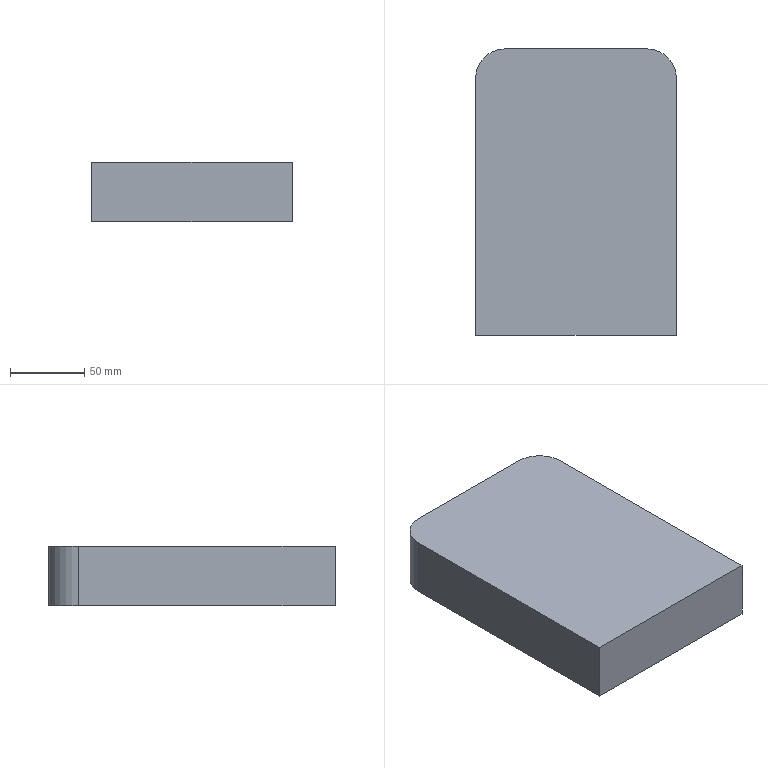Part | SolidWorks | features Extrusion 1, Shell 1 | 1 solid | 15 faces | box 135.332 x 192.723 x 40 mm | volume 238240 mm3 | plane 11 | cylinder 4 | commonest cylinder face diameters 30 x2 40 x2
STEP:
#1=CARTESIAN_POINT('',(-11.593,120.781,0.));
#2=VERTEX_POINT('',#1);
#3=CARTESIAN_POINT('',(-11.593,-51.942,0.));
#4=VERTEX_POINT('',#3);
#5=CARTESIAN_POINT('',(-11.593,120.781,0.));
#6=DIRECTION('',(0.,-1.,0.));
#7=VECTOR('',#6,1000.);
#8=LINE('',#5,#7);
#9=EDGE_CURVE('',#2,#4,#8,.T.);
#10=ORIENTED_EDGE('',*,*,#9,.T.);
#11=CARTESIAN_POINT('',(-11.593,-51.942,40.));
#12=VERTEX_POINT('',#11);
#13=CARTESIAN_POINT('',(-11.593,-51.942,40.));
#14=DIRECTION('',(0.,0.,-1.));
#15=VECTOR('',#14,1000.);
#16=LINE('',#13,#15);
#17=EDGE_CURVE('',#12,#4,#16,.T.);
#18=ORIENTED_EDGE('',*,*,#17,.F.);
#19=CARTESIAN_POINT('',(-11.593,120.781,40.));
#20=VERTEX_POINT('',#19);
#21=CARTESIAN_POINT('',(-11.593,120.781,40.));
#22=DIRECTION('',(0.,-1.,0.));
#23=VECTOR('',#22,1000.);
#24=LINE('',#21,#23);
#25=EDGE_CURVE('',#20,#12,#24,.T.);
#26=ORIENTED_EDGE('',*,*,#25,.F.);
#27=CARTESIAN_POINT('',(-11.593,120.781,40.));
#28=DIRECTION('',(0.,0.,-1.));
#29=VECTOR('',#28,1000.);
#30=LINE('',#27,#29);
#31=EDGE_CURVE('',#20,#2,#30,.T.);
#32=ORIENTED_EDGE('',*,*,#31,.T.);
#33=EDGE_LOOP('',(#10,#18,#26,#32));
#34=FACE_OUTER_BOUND('',#33,.T.);
#35=CARTESIAN_POINT('',(-11.593,120.781,40.));
#36=DIRECTION('',(1.,0.,0.));
#37=DIRECTION('',(0.,1.,0.));
#38=AXIS2_PLACEMENT_3D('',#35,#36,#37);
#39=PLANE('',#38);
#40=ADVANCED_FACE('',(#34),#39,.F.);
#41=CARTESIAN_POINT('',(123.739,-51.942,0.));
#42=VERTEX_POINT('',#41);
#43=CARTESIAN_POINT('',(92.171,-51.942,0.));
#44=DIRECTION('',(1.,0.,0.));
#45=VECTOR('',#44,1000.);
#46=LINE('',#43,#45);
#47=EDGE_CURVE('',#4,#42,#46,.T.);
#48=ORIENTED_EDGE('',*,*,#47,.T.);
#49=CARTESIAN_POINT('',(123.739,-51.942,40.));
#50=VERTEX_POINT('',#49);
#51=CARTESIAN_POINT('',(123.739,-51.942,40.));
#52=DIRECTION('',(0.,0.,-1.));
#53=VECTOR('',#52,1000.);
#54=LINE('',#51,#53);
#55=EDGE_CURVE('',#50,#42,#54,.T.);
#56=ORIENTED_EDGE('',*,*,#55,.F.);
#57=CARTESIAN_POINT('',(-11.593,-51.942,40.));
#58=DIRECTION('',(1.,0.,0.));
#59=VECTOR('',#58,1000.);
#60=LINE('',#57,#59);
#61=EDGE_CURVE('',#12,#50,#60,.T.);
#62=ORIENTED_EDGE('',*,*,#61,.F.);
#63=ORIENTED_EDGE('',*,*,#17,.T.);
#64=EDGE_LOOP('',(#48,#56,#62,#63));
#65=FACE_OUTER_BOUND('',#64,.T.);
#66=CARTESIAN_POINT('',(92.171,-51.942,40.));
#67=DIRECTION('',(0.,1.,0.));
#68=DIRECTION('',(0.,0.,1.));
#69=AXIS2_PLACEMENT_3D('',#66,#67,#68);
#70=PLANE('',#69);
#71=ADVANCED_FACE('',(#65),#70,.F.);
#72=CARTESIAN_POINT('',(123.739,120.781,0.));
#73=VERTEX_POINT('',#72);
#74=CARTESIAN_POINT('',(123.739,-51.942,0.));
#75=DIRECTION('',(0.,1.,0.));
#76=VECTOR('',#75,1000.);
#77=LINE('',#74,#76);
#78=EDGE_CURVE('',#42,#73,#77,.T.);
#79=ORIENTED_EDGE('',*,*,#78,.T.);
#80=CARTESIAN_POINT('',(123.739,120.781,40.));
#81=VERTEX_POINT('',#80);
#82=CARTESIAN_POINT('',(123.739,120.781,40.));
#83=DIRECTION('',(0.,0.,-1.));
#84=VECTOR('',#83,1000.);
#85=LINE('',#82,#84);
#86=EDGE_CURVE('',#81,#73,#85,.T.);
#87=ORIENTED_EDGE('',*,*,#86,.F.);
#88=CARTESIAN_POINT('',(123.739,-51.942,40.));
#89=DIRECTION('',(0.,1.,0.));
#90=VECTOR('',#89,1000.);
#91=LINE('',#88,#90);
#92=EDGE_CURVE('',#50,#81,#91,.T.);
#93=ORIENTED_EDGE('',*,*,#92,.F.);
#94=ORIENTED_EDGE('',*,*,#55,.T.);
#95=EDGE_LOOP('',(#79,#87,#93,#94));
#96=FACE_OUTER_BOUND('',#95,.T.);
#97=CARTESIAN_POINT('',(123.739,-51.942,40.));
#98=DIRECTION('',(-1.,0.,0.));
#99=DIRECTION('',(0.,-1.,0.));
#100=AXIS2_PLACEMENT_3D('',#97,#98,#99);
#101=PLANE('',#100);
#102=ADVANCED_FACE('',(#96),#101,.F.);
#103=CARTESIAN_POINT('',(103.739,140.781,0.));
#104=VERTEX_POINT('',#103);
#105=CARTESIAN_POINT('',(103.739,120.781,0.));
#106=DIRECTION('',(0.,0.,1.));
#107=DIRECTION('',(1.,0.,0.));
#108=AXIS2_PLACEMENT_3D('',#105,#106,#107);
#109=CIRCLE('',#108,20.);
#110=EDGE_CURVE('',#73,#104,#109,.T.);
#111=ORIENTED_EDGE('',*,*,#110,.T.);
#112=CARTESIAN_POINT('',(103.739,140.781,40.));
#113=VERTEX_POINT('',#112);
#114=CARTESIAN_POINT('',(103.739,140.781,40.));
#115=DIRECTION('',(0.,0.,-1.));
#116=VECTOR('',#115,1000.);
#117=LINE('',#114,#116);
#118=EDGE_CURVE('',#113,#104,#117,.T.);
#119=ORIENTED_EDGE('',*,*,#118,.F.);
#120=CARTESIAN_POINT('',(103.739,120.781,40.));
#121=DIRECTION('',(0.,0.,1.));
#122=DIRECTION('',(1.,0.,0.));
#123=AXIS2_PLACEMENT_3D('',#120,#121,#122);
#124=CIRCLE('',#123,20.);
#125=EDGE_CURVE('',#81,#113,#124,.T.);
#126=ORIENTED_EDGE('',*,*,#125,.F.);
#127=ORIENTED_EDGE('',*,*,#86,.T.);
#128=EDGE_LOOP('',(#111,#119,#126,#127));
#129=FACE_OUTER_BOUND('',#128,.T.);
#130=CARTESIAN_POINT('',(103.739,120.781,40.));
#131=DIRECTION('',(0.,0.,-1.));
#132=DIRECTION('',(-1.,0.,0.));
#133=AXIS2_PLACEMENT_3D('',#130,#131,#132);
#134=CYLINDRICAL_SURFACE('',#133,20.);
#135=ADVANCED_FACE('',(#129),#134,.T.);
#136=CARTESIAN_POINT('',(8.407,140.781,0.));
#137=VERTEX_POINT('',#136);
#138=CARTESIAN_POINT('',(103.739,140.781,0.));
#139=DIRECTION('',(-1.,0.,0.));
#140=VECTOR('',#139,1000.);
#141=LINE('',#138,#140);
#142=EDGE_CURVE('',#104,#137,#141,.T.);
#143=ORIENTED_EDGE('',*,*,#142,.T.);
#144=CARTESIAN_POINT('',(8.407,140.781,40.));
#145=VERTEX_POINT('',#144);
#146=CARTESIAN_POINT('',(8.407,140.781,40.));
#147=DIRECTION('',(0.,0.,-1.));
#148=VECTOR('',#147,1000.);
#149=LINE('',#146,#148);
#150=EDGE_CURVE('',#145,#137,#149,.T.);
#151=ORIENTED_EDGE('',*,*,#150,.F.);
#152=CARTESIAN_POINT('',(103.739,140.781,40.));
#153=DIRECTION('',(-1.,0.,0.));
#154=VECTOR('',#153,1000.);
#155=LINE('',#152,#154);
#156=EDGE_CURVE('',#113,#145,#155,.T.);
#157=ORIENTED_EDGE('',*,*,#156,.F.);
#158=ORIENTED_EDGE('',*,*,#118,.T.);
#159=EDGE_LOOP('',(#143,#151,#157,#158));
#160=FACE_OUTER_BOUND('',#159,.T.);
#161=CARTESIAN_POINT('',(103.739,140.781,40.));
#162=DIRECTION('',(0.,-1.,0.));
#163=DIRECTION('',(0.,0.,-1.));
#164=AXIS2_PLACEMENT_3D('',#161,#162,#163);
#165=PLANE('',#164);
#166=ADVANCED_FACE('',(#160),#165,.F.);
#167=CARTESIAN_POINT('',(8.407,120.781,0.));
#168=DIRECTION('',(0.,0.,1.));
#169=DIRECTION('',(1.,0.,0.));
#170=AXIS2_PLACEMENT_3D('',#167,#168,#169);
#171=CIRCLE('',#170,20.);
#172=EDGE_CURVE('',#137,#2,#171,.T.);
#173=ORIENTED_EDGE('',*,*,#172,.T.);
#174=ORIENTED_EDGE('',*,*,#31,.F.);
#175=CARTESIAN_POINT('',(8.407,120.781,40.));
#176=DIRECTION('',(0.,0.,1.));
#177=DIRECTION('',(1.,0.,0.));
#178=AXIS2_PLACEMENT_3D('',#175,#176,#177);
#179=CIRCLE('',#178,20.);
#180=EDGE_CURVE('',#145,#20,#179,.T.);
#181=ORIENTED_EDGE('',*,*,#180,.F.);
#182=ORIENTED_EDGE('',*,*,#150,.T.);
#183=EDGE_LOOP('',(#173,#174,#181,#182));
#184=FACE_OUTER_BOUND('',#183,.T.);
#185=CARTESIAN_POINT('',(8.407,120.781,40.));
#186=DIRECTION('',(0.,0.,-1.));
#187=DIRECTION('',(-1.,0.,0.));
#188=AXIS2_PLACEMENT_3D('',#185,#186,#187);
#189=CYLINDRICAL_SURFACE('',#188,20.);
#190=ADVANCED_FACE('',(#184),#189,.T.);
#191=ORIENTED_EDGE('',*,*,#25,.T.);
#192=ORIENTED_EDGE('',*,*,#61,.T.);
#193=ORIENTED_EDGE('',*,*,#92,.T.);
#194=ORIENTED_EDGE('',*,*,#125,.T.);
#195=ORIENTED_EDGE('',*,*,#156,.T.);
#196=ORIENTED_EDGE('',*,*,#180,.T.);
#197=EDGE_LOOP('',(#191,#192,#193,#194,#195,#196));
#198=FACE_OUTER_BOUND('',#197,.T.);
#199=CARTESIAN_POINT('',(103.739,120.781,40.));
#200=DIRECTION('',(0.,0.,1.));
#201=DIRECTION('',(1.,0.,0.));
#202=AXIS2_PLACEMENT_3D('',#199,#200,#201);
#203=PLANE('',#202);
#204=ADVANCED_FACE('',(#198),#203,.T.);
#205=CARTESIAN_POINT('',(8.407,135.781,0.));
#206=VERTEX_POINT('',#205);
#207=CARTESIAN_POINT('',(-6.593,120.781,0.));
#208=VERTEX_POINT('',#207);
#209=CARTESIAN_POINT('',(8.407,120.781,0.));
#210=DIRECTION('',(0.,0.,1.));
#211=DIRECTION('',(1.,0.,0.));
#212=AXIS2_PLACEMENT_3D('',#209,#210,#211);
#213=CIRCLE('',#212,15.);
#214=EDGE_CURVE('',#206,#208,#213,.T.);
#215=ORIENTED_EDGE('',*,*,#214,.T.);
#216=CARTESIAN_POINT('',(-6.593,-46.942,0.));
#217=VERTEX_POINT('',#216);
#218=CARTESIAN_POINT('',(-6.593,120.781,0.));
#219=DIRECTION('',(0.,-1.,0.));
#220=VECTOR('',#219,1000.);
#221=LINE('',#218,#220);
#222=EDGE_CURVE('',#208,#217,#221,.T.);
#223=ORIENTED_EDGE('',*,*,#222,.T.);
#224=CARTESIAN_POINT('',(118.739,-46.942,0.));
#225=VERTEX_POINT('',#224);
#226=CARTESIAN_POINT('',(92.171,-46.942,0.));
#227=DIRECTION('',(1.,0.,0.));
#228=VECTOR('',#227,1000.);
#229=LINE('',#226,#228);
#230=EDGE_CURVE('',#217,#225,#229,.T.);
#231=ORIENTED_EDGE('',*,*,#230,.T.);
#232=CARTESIAN_POINT('',(118.739,120.781,0.));
#233=VERTEX_POINT('',#232);
#234=CARTESIAN_POINT('',(118.739,-51.942,0.));
#235=DIRECTION('',(0.,1.,0.));
#236=VECTOR('',#235,1000.);
#237=LINE('',#234,#236);
#238=EDGE_CURVE('',#225,#233,#237,.T.);
#239=ORIENTED_EDGE('',*,*,#238,.T.);
#240=CARTESIAN_POINT('',(103.739,135.781,0.));
#241=VERTEX_POINT('',#240);
#242=CARTESIAN_POINT('',(103.739,120.781,0.));
#243=DIRECTION('',(0.,0.,1.));
#244=DIRECTION('',(1.,0.,0.));
#245=AXIS2_PLACEMENT_3D('',#242,#243,#244);
#246=CIRCLE('',#245,15.);
#247=EDGE_CURVE('',#233,#241,#246,.T.);
#248=ORIENTED_EDGE('',*,*,#247,.T.);
#249=CARTESIAN_POINT('',(103.739,135.781,0.));
#250=DIRECTION('',(-1.,0.,0.));
#251=VECTOR('',#250,1000.);
#252=LINE('',#249,#251);
#253=EDGE_CURVE('',#241,#206,#252,.T.);
#254=ORIENTED_EDGE('',*,*,#253,.T.);
#255=EDGE_LOOP('',(#215,#223,#231,#239,#248,#254));
#256=FACE_BOUND('',#255,.T.);
#257=ORIENTED_EDGE('',*,*,#9,.F.);
#258=ORIENTED_EDGE('',*,*,#172,.F.);
#259=ORIENTED_EDGE('',*,*,#142,.F.);
#260=ORIENTED_EDGE('',*,*,#110,.F.);
#261=ORIENTED_EDGE('',*,*,#78,.F.);
#262=ORIENTED_EDGE('',*,*,#47,.F.);
#263=EDGE_LOOP('',(#257,#258,#259,#260,#261,#262));
#264=FACE_OUTER_BOUND('',#263,.T.);
#265=CARTESIAN_POINT('',(103.739,120.781,0.));
#266=DIRECTION('',(0.,0.,1.));
#267=DIRECTION('',(1.,0.,0.));
#268=AXIS2_PLACEMENT_3D('',#265,#266,#267);
#269=PLANE('',#268);
#270=ADVANCED_FACE('',(#256,#264),#269,.F.);
#271=ORIENTED_EDGE('',*,*,#222,.F.);
#272=CARTESIAN_POINT('',(-6.593,120.781,35.));
#273=VERTEX_POINT('',#272);
#274=CARTESIAN_POINT('',(-6.593,120.781,40.));
#275=DIRECTION('',(0.,0.,-1.));
#276=VECTOR('',#275,1000.);
#277=LINE('',#274,#276);
#278=EDGE_CURVE('',#273,#208,#277,.T.);
#279=ORIENTED_EDGE('',*,*,#278,.F.);
#280=CARTESIAN_POINT('',(-6.593,-46.942,35.));
#281=VERTEX_POINT('',#280);
#282=CARTESIAN_POINT('',(-6.593,120.781,35.));
#283=DIRECTION('',(0.,-1.,0.));
#284=VECTOR('',#283,1000.);
#285=LINE('',#282,#284);
#286=EDGE_CURVE('',#273,#281,#285,.T.);
#287=ORIENTED_EDGE('',*,*,#286,.T.);
#288=CARTESIAN_POINT('',(-6.593,-46.942,40.));
#289=DIRECTION('',(0.,0.,-1.));
#290=VECTOR('',#289,1000.);
#291=LINE('',#288,#290);
#292=EDGE_CURVE('',#281,#217,#291,.T.);
#293=ORIENTED_EDGE('',*,*,#292,.T.);
#294=EDGE_LOOP('',(#271,#279,#287,#293));
#295=FACE_OUTER_BOUND('',#294,.T.);
#296=CARTESIAN_POINT('',(-6.593,120.781,40.));
#297=DIRECTION('',(1.,0.,0.));
#298=DIRECTION('',(0.,1.,0.));
#299=AXIS2_PLACEMENT_3D('',#296,#297,#298);
#300=PLANE('',#299);
#301=ADVANCED_FACE('',(#295),#300,.T.);
#302=ORIENTED_EDGE('',*,*,#230,.F.);
#303=ORIENTED_EDGE('',*,*,#292,.F.);
#304=CARTESIAN_POINT('',(118.739,-46.942,35.));
#305=VERTEX_POINT('',#304);
#306=CARTESIAN_POINT('',(92.171,-46.942,35.));
#307=DIRECTION('',(1.,0.,0.));
#308=VECTOR('',#307,1000.);
#309=LINE('',#306,#308);
#310=EDGE_CURVE('',#281,#305,#309,.T.);
#311=ORIENTED_EDGE('',*,*,#310,.T.);
#312=CARTESIAN_POINT('',(118.739,-46.942,40.));
#313=DIRECTION('',(0.,0.,-1.));
#314=VECTOR('',#313,1000.);
#315=LINE('',#312,#314);
#316=EDGE_CURVE('',#305,#225,#315,.T.);
#317=ORIENTED_EDGE('',*,*,#316,.T.);
#318=EDGE_LOOP('',(#302,#303,#311,#317));
#319=FACE_OUTER_BOUND('',#318,.T.);
#320=CARTESIAN_POINT('',(92.171,-46.942,40.));
#321=DIRECTION('',(0.,1.,0.));
#322=DIRECTION('',(0.,0.,1.));
#323=AXIS2_PLACEMENT_3D('',#320,#321,#322);
#324=PLANE('',#323);
#325=ADVANCED_FACE('',(#319),#324,.T.);
#326=ORIENTED_EDGE('',*,*,#238,.F.);
#327=ORIENTED_EDGE('',*,*,#316,.F.);
#328=CARTESIAN_POINT('',(118.739,120.781,35.));
#329=VERTEX_POINT('',#328);
#330=CARTESIAN_POINT('',(118.739,-51.942,35.));
#331=DIRECTION('',(0.,1.,0.));
#332=VECTOR('',#331,1000.);
#333=LINE('',#330,#332);
#334=EDGE_CURVE('',#305,#329,#333,.T.);
#335=ORIENTED_EDGE('',*,*,#334,.T.);
#336=CARTESIAN_POINT('',(118.739,120.781,40.));
#337=DIRECTION('',(0.,0.,-1.));
#338=VECTOR('',#337,1000.);
#339=LINE('',#336,#338);
#340=EDGE_CURVE('',#329,#233,#339,.T.);
#341=ORIENTED_EDGE('',*,*,#340,.T.);
#342=EDGE_LOOP('',(#326,#327,#335,#341));
#343=FACE_OUTER_BOUND('',#342,.T.);
#344=CARTESIAN_POINT('',(118.739,-51.942,40.));
#345=DIRECTION('',(-1.,0.,0.));
#346=DIRECTION('',(0.,-1.,0.));
#347=AXIS2_PLACEMENT_3D('',#344,#345,#346);
#348=PLANE('',#347);
#349=ADVANCED_FACE('',(#343),#348,.T.);
#350=ORIENTED_EDGE('',*,*,#247,.F.);
#351=ORIENTED_EDGE('',*,*,#340,.F.);
#352=CARTESIAN_POINT('',(103.739,135.781,35.));
#353=VERTEX_POINT('',#352);
#354=CARTESIAN_POINT('',(103.739,120.781,35.));
#355=DIRECTION('',(0.,0.,1.));
#356=DIRECTION('',(1.,0.,0.));
#357=AXIS2_PLACEMENT_3D('',#354,#355,#356);
#358=CIRCLE('',#357,15.);
#359=EDGE_CURVE('',#329,#353,#358,.T.);
#360=ORIENTED_EDGE('',*,*,#359,.T.);
#361=CARTESIAN_POINT('',(103.739,135.781,40.));
#362=DIRECTION('',(0.,0.,-1.));
#363=VECTOR('',#362,1000.);
#364=LINE('',#361,#363);
#365=EDGE_CURVE('',#353,#241,#364,.T.);
#366=ORIENTED_EDGE('',*,*,#365,.T.);
#367=EDGE_LOOP('',(#350,#351,#360,#366));
#368=FACE_OUTER_BOUND('',#367,.T.);
#369=CARTESIAN_POINT('',(103.739,120.781,40.));
#370=DIRECTION('',(0.,0.,-1.));
#371=DIRECTION('',(-1.,0.,0.));
#372=AXIS2_PLACEMENT_3D('',#369,#370,#371);
#373=CYLINDRICAL_SURFACE('',#372,15.);
#374=ADVANCED_FACE('',(#368),#373,.F.);
#375=ORIENTED_EDGE('',*,*,#253,.F.);
#376=ORIENTED_EDGE('',*,*,#365,.F.);
#377=CARTESIAN_POINT('',(8.407,135.781,35.));
#378=VERTEX_POINT('',#377);
#379=CARTESIAN_POINT('',(103.739,135.781,35.));
#380=DIRECTION('',(-1.,0.,0.));
#381=VECTOR('',#380,1000.);
#382=LINE('',#379,#381);
#383=EDGE_CURVE('',#353,#378,#382,.T.);
#384=ORIENTED_EDGE('',*,*,#383,.T.);
#385=CARTESIAN_POINT('',(8.407,135.781,40.));
#386=DIRECTION('',(0.,0.,-1.));
#387=VECTOR('',#386,1000.);
#388=LINE('',#385,#387);
#389=EDGE_CURVE('',#378,#206,#388,.T.);
#390=ORIENTED_EDGE('',*,*,#389,.T.);
#391=EDGE_LOOP('',(#375,#376,#384,#390));
#392=FACE_OUTER_BOUND('',#391,.T.);
#393=CARTESIAN_POINT('',(103.739,135.781,40.));
#394=DIRECTION('',(0.,-1.,0.));
#395=DIRECTION('',(0.,0.,-1.));
#396=AXIS2_PLACEMENT_3D('',#393,#394,#395);
#397=PLANE('',#396);
#398=ADVANCED_FACE('',(#392),#397,.T.);
#399=ORIENTED_EDGE('',*,*,#214,.F.);
#400=ORIENTED_EDGE('',*,*,#389,.F.);
#401=CARTESIAN_POINT('',(8.407,120.781,35.));
#402=DIRECTION('',(0.,0.,1.));
#403=DIRECTION('',(1.,0.,0.));
#404=AXIS2_PLACEMENT_3D('',#401,#402,#403);
#405=CIRCLE('',#404,15.);
#406=EDGE_CURVE('',#378,#273,#405,.T.);
#407=ORIENTED_EDGE('',*,*,#406,.T.);
#408=ORIENTED_EDGE('',*,*,#278,.T.);
#409=EDGE_LOOP('',(#399,#400,#407,#408));
#410=FACE_OUTER_BOUND('',#409,.T.);
#411=CARTESIAN_POINT('',(8.407,120.781,40.));
#412=DIRECTION('',(0.,0.,-1.));
#413=DIRECTION('',(-1.,0.,0.));
#414=AXIS2_PLACEMENT_3D('',#411,#412,#413);
#415=CYLINDRICAL_SURFACE('',#414,15.);
#416=ADVANCED_FACE('',(#410),#415,.F.);
#417=ORIENTED_EDGE('',*,*,#286,.F.);
#418=ORIENTED_EDGE('',*,*,#406,.F.);
#419=ORIENTED_EDGE('',*,*,#383,.F.);
#420=ORIENTED_EDGE('',*,*,#359,.F.);
#421=ORIENTED_EDGE('',*,*,#334,.F.);
#422=ORIENTED_EDGE('',*,*,#310,.F.);
#423=EDGE_LOOP('',(#417,#418,#419,#420,#421,#422));
#424=FACE_OUTER_BOUND('',#423,.T.);
#425=CARTESIAN_POINT('',(103.739,120.781,35.));
#426=DIRECTION('',(0.,0.,1.));
#427=DIRECTION('',(1.,0.,0.));
#428=AXIS2_PLACEMENT_3D('',#425,#426,#427);
#429=PLANE('',#428);
#430=ADVANCED_FACE('',(#424),#429,.F.);
#431=CLOSED_SHELL('',(#40,#71,#102,#135,#166,#190,#204,#270,#301,#325,#349,#374,#398,#416,#430));
#432=MANIFOLD_SOLID_BREP('',#431);
#433=CARTESIAN_POINT('',(0.,0.,0.));
#434=DIRECTION('',(0.,0.,1.));
#435=DIRECTION('',(1.,0.,0.));
#436=AXIS2_PLACEMENT_3D('',#433,#434,#435);
#437=(LENGTH_UNIT()NAMED_UNIT(*)SI_UNIT(.MILLI.,.METRE.));
#438=UNCERTAINTY_MEASURE_WITH_UNIT(LENGTH_MEASURE(0.00001),#437,'','');
#439=(NAMED_UNIT(*)PLANE_ANGLE_UNIT()SI_UNIT($,.RADIAN.));
#440=(NAMED_UNIT(*)SI_UNIT($,.STERADIAN.)SOLID_ANGLE_UNIT());
#441=(GEOMETRIC_REPRESENTATION_CONTEXT(3)GLOBAL_UNCERTAINTY_ASSIGNED_CONTEXT((#438))GLOBAL_UNIT_ASSIGNED_CONTEXT((#437,#439,#440))REPRESENTATION_CONTEXT('',''));
#442=ADVANCED_BREP_SHAPE_REPRESENTATION('',(#432,#436),#441);